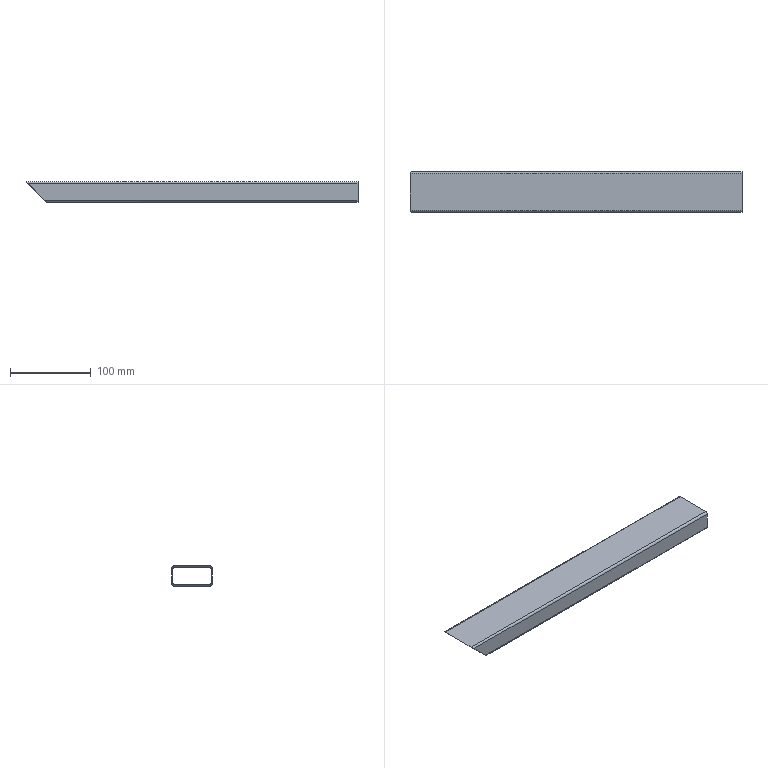Part | STEP file | 6150501 | 1 solid | 18 faces | box 410 x 50 x 25 mm | volume 84495 mm3 | plane 10 | cylinder 8 | commonest cylinder face diameters 3 x4 5 x4
STEP:
#1=CARTESIAN_POINT('',(205.,-25.,10.));
#2=VERTEX_POINT('',#1);
#3=CARTESIAN_POINT('',(-202.5,-25.,10.));
#4=VERTEX_POINT('',#3);
#5=CARTESIAN_POINT('',(-205.,-25.,10.));
#6=DIRECTION('',(-1.,0.,0.));
#7=VECTOR('',#6,1000.);
#8=LINE('',#5,#7);
#9=EDGE_CURVE('',#2,#4,#8,.T.);
#10=ORIENTED_EDGE('',*,*,#9,.T.);
#11=CARTESIAN_POINT('',(-182.5,-25.,-10.));
#12=VERTEX_POINT('',#11);
#13=CARTESIAN_POINT('',(-205.,-25.,12.5));
#14=DIRECTION('',(0.7071,0.,-0.7071));
#15=VECTOR('',#14,1000.);
#16=LINE('',#13,#15);
#17=EDGE_CURVE('',#4,#12,#16,.T.);
#18=ORIENTED_EDGE('',*,*,#17,.T.);
#19=CARTESIAN_POINT('',(205.,-25.,-10.));
#20=VERTEX_POINT('',#19);
#21=CARTESIAN_POINT('',(-205.,-25.,-10.));
#22=DIRECTION('',(1.,0.,0.));
#23=VECTOR('',#22,1000.);
#24=LINE('',#21,#23);
#25=EDGE_CURVE('',#12,#20,#24,.T.);
#26=ORIENTED_EDGE('',*,*,#25,.T.);
#27=CARTESIAN_POINT('',(205.,-25.,12.5));
#28=DIRECTION('',(0.,0.,-1.));
#29=VECTOR('',#28,1000.);
#30=LINE('',#27,#29);
#31=EDGE_CURVE('',#2,#20,#30,.T.);
#32=ORIENTED_EDGE('',*,*,#31,.F.);
#33=EDGE_LOOP('',(#10,#18,#26,#32));
#34=FACE_OUTER_BOUND('',#33,.T.);
#35=CARTESIAN_POINT('',(-205.,-25.,12.5));
#36=DIRECTION('',(0.,1.,0.));
#37=DIRECTION('',(-1.,0.,0.));
#38=AXIS2_PLACEMENT_3D('',#35,#36,#37);
#39=PLANE('',#38);
#40=ADVANCED_FACE('',(#34),#39,.F.);
#41=CARTESIAN_POINT('',(205.,-22.,-11.));
#42=VERTEX_POINT('',#41);
#43=CARTESIAN_POINT('',(205.,22.,-11.));
#44=VERTEX_POINT('',#43);
#45=CARTESIAN_POINT('',(205.,22.,-11.));
#46=DIRECTION('',(0.,1.,0.));
#47=VECTOR('',#46,1000.);
#48=LINE('',#45,#47);
#49=EDGE_CURVE('',#42,#44,#48,.T.);
#50=ORIENTED_EDGE('',*,*,#49,.F.);
#51=CARTESIAN_POINT('',(205.,-23.5,-9.5));
#52=VERTEX_POINT('',#51);
#53=CARTESIAN_POINT('',(205.,-22.,-9.5));
#54=DIRECTION('',(1.,0.,0.));
#55=DIRECTION('',(0.,0.,-1.));
#56=AXIS2_PLACEMENT_3D('',#53,#54,#55);
#57=CIRCLE('',#56,1.5);
#58=EDGE_CURVE('',#52,#42,#57,.T.);
#59=ORIENTED_EDGE('',*,*,#58,.F.);
#60=CARTESIAN_POINT('',(205.,-23.5,9.5));
#61=VERTEX_POINT('',#60);
#62=CARTESIAN_POINT('',(205.,-23.5,9.5));
#63=DIRECTION('',(0.,0.,-1.));
#64=VECTOR('',#63,1000.);
#65=LINE('',#62,#64);
#66=EDGE_CURVE('',#61,#52,#65,.T.);
#67=ORIENTED_EDGE('',*,*,#66,.F.);
#68=CARTESIAN_POINT('',(205.,-22.,11.));
#69=VERTEX_POINT('',#68);
#70=CARTESIAN_POINT('',(205.,-22.,9.5));
#71=DIRECTION('',(1.,0.,0.));
#72=DIRECTION('',(0.,0.,-1.));
#73=AXIS2_PLACEMENT_3D('',#70,#71,#72);
#74=CIRCLE('',#73,1.5);
#75=EDGE_CURVE('',#69,#61,#74,.T.);
#76=ORIENTED_EDGE('',*,*,#75,.F.);
#77=CARTESIAN_POINT('',(205.,22.,11.));
#78=VERTEX_POINT('',#77);
#79=CARTESIAN_POINT('',(205.,22.,11.));
#80=DIRECTION('',(0.,-1.,0.));
#81=VECTOR('',#80,1000.);
#82=LINE('',#79,#81);
#83=EDGE_CURVE('',#78,#69,#82,.T.);
#84=ORIENTED_EDGE('',*,*,#83,.F.);
#85=CARTESIAN_POINT('',(205.,23.5,9.5));
#86=VERTEX_POINT('',#85);
#87=CARTESIAN_POINT('',(205.,22.,9.5));
#88=DIRECTION('',(1.,0.,0.));
#89=DIRECTION('',(0.,0.,-1.));
#90=AXIS2_PLACEMENT_3D('',#87,#88,#89);
#91=CIRCLE('',#90,1.5);
#92=EDGE_CURVE('',#86,#78,#91,.T.);
#93=ORIENTED_EDGE('',*,*,#92,.F.);
#94=CARTESIAN_POINT('',(205.,23.5,-9.5));
#95=VERTEX_POINT('',#94);
#96=CARTESIAN_POINT('',(205.,23.5,9.5));
#97=DIRECTION('',(0.,0.,1.));
#98=VECTOR('',#97,1000.);
#99=LINE('',#96,#98);
#100=EDGE_CURVE('',#95,#86,#99,.T.);
#101=ORIENTED_EDGE('',*,*,#100,.F.);
#102=CARTESIAN_POINT('',(205.,22.,-9.5));
#103=DIRECTION('',(1.,0.,0.));
#104=DIRECTION('',(0.,0.,1.));
#105=AXIS2_PLACEMENT_3D('',#102,#103,#104);
#106=CIRCLE('',#105,1.5);
#107=EDGE_CURVE('',#44,#95,#106,.T.);
#108=ORIENTED_EDGE('',*,*,#107,.F.);
#109=EDGE_LOOP('',(#50,#59,#67,#76,#84,#93,#101,#108));
#110=FACE_BOUND('',#109,.T.);
#111=CARTESIAN_POINT('',(205.,-22.5,12.5));
#112=VERTEX_POINT('',#111);
#113=CARTESIAN_POINT('',(205.,22.5,12.5));
#114=VERTEX_POINT('',#113);
#115=CARTESIAN_POINT('',(205.,25.,12.5));
#116=DIRECTION('',(0.,1.,0.));
#117=VECTOR('',#116,1000.);
#118=LINE('',#115,#117);
#119=EDGE_CURVE('',#112,#114,#118,.T.);
#120=ORIENTED_EDGE('',*,*,#119,.F.);
#121=CARTESIAN_POINT('',(205.,-22.5,10.));
#122=DIRECTION('',(1.,0.,0.));
#123=DIRECTION('',(0.,0.,1.));
#124=AXIS2_PLACEMENT_3D('',#121,#122,#123);
#125=CIRCLE('',#124,2.5);
#126=EDGE_CURVE('',#112,#2,#125,.T.);
#127=ORIENTED_EDGE('',*,*,#126,.T.);
#128=ORIENTED_EDGE('',*,*,#31,.T.);
#129=CARTESIAN_POINT('',(205.,-22.5,-12.5));
#130=VERTEX_POINT('',#129);
#131=CARTESIAN_POINT('',(205.,-22.5,-10.));
#132=DIRECTION('',(1.,0.,0.));
#133=DIRECTION('',(0.,0.,1.));
#134=AXIS2_PLACEMENT_3D('',#131,#132,#133);
#135=CIRCLE('',#134,2.5);
#136=EDGE_CURVE('',#20,#130,#135,.T.);
#137=ORIENTED_EDGE('',*,*,#136,.T.);
#138=CARTESIAN_POINT('',(205.,22.5,-12.5));
#139=VERTEX_POINT('',#138);
#140=CARTESIAN_POINT('',(205.,25.,-12.5));
#141=DIRECTION('',(0.,1.,0.));
#142=VECTOR('',#141,1000.);
#143=LINE('',#140,#142);
#144=EDGE_CURVE('',#130,#139,#143,.T.);
#145=ORIENTED_EDGE('',*,*,#144,.T.);
#146=CARTESIAN_POINT('',(205.,25.,-10.));
#147=VERTEX_POINT('',#146);
#148=CARTESIAN_POINT('',(205.,22.5,-10.));
#149=DIRECTION('',(1.,0.,0.));
#150=DIRECTION('',(0.,0.,1.));
#151=AXIS2_PLACEMENT_3D('',#148,#149,#150);
#152=CIRCLE('',#151,2.5);
#153=EDGE_CURVE('',#139,#147,#152,.T.);
#154=ORIENTED_EDGE('',*,*,#153,.T.);
#155=CARTESIAN_POINT('',(205.,25.,10.));
#156=VERTEX_POINT('',#155);
#157=CARTESIAN_POINT('',(205.,25.,12.5));
#158=DIRECTION('',(0.,0.,-1.));
#159=VECTOR('',#158,1000.);
#160=LINE('',#157,#159);
#161=EDGE_CURVE('',#156,#147,#160,.T.);
#162=ORIENTED_EDGE('',*,*,#161,.F.);
#163=CARTESIAN_POINT('',(205.,22.5,10.));
#164=DIRECTION('',(1.,0.,0.));
#165=DIRECTION('',(0.,0.,1.));
#166=AXIS2_PLACEMENT_3D('',#163,#164,#165);
#167=CIRCLE('',#166,2.5);
#168=EDGE_CURVE('',#156,#114,#167,.T.);
#169=ORIENTED_EDGE('',*,*,#168,.T.);
#170=EDGE_LOOP('',(#120,#127,#128,#137,#145,#154,#162,#169));
#171=FACE_OUTER_BOUND('',#170,.T.);
#172=CARTESIAN_POINT('',(205.,25.,12.5));
#173=DIRECTION('',(-1.,0.,0.));
#174=DIRECTION('',(0.,0.,1.));
#175=AXIS2_PLACEMENT_3D('',#172,#173,#174);
#176=PLANE('',#175);
#177=ADVANCED_FACE('',(#110,#171),#176,.F.);
#178=CARTESIAN_POINT('',(-182.5,25.,-10.));
#179=VERTEX_POINT('',#178);
#180=CARTESIAN_POINT('',(-205.,25.,-10.));
#181=DIRECTION('',(-1.,0.,0.));
#182=VECTOR('',#181,1000.);
#183=LINE('',#180,#182);
#184=EDGE_CURVE('',#147,#179,#183,.T.);
#185=ORIENTED_EDGE('',*,*,#184,.T.);
#186=CARTESIAN_POINT('',(-202.5,25.,10.));
#187=VERTEX_POINT('',#186);
#188=CARTESIAN_POINT('',(-205.,25.,12.5));
#189=DIRECTION('',(0.7071,0.,-0.7071));
#190=VECTOR('',#189,1000.);
#191=LINE('',#188,#190);
#192=EDGE_CURVE('',#187,#179,#191,.T.);
#193=ORIENTED_EDGE('',*,*,#192,.F.);
#194=CARTESIAN_POINT('',(205.,25.,10.));
#195=DIRECTION('',(1.,0.,0.));
#196=VECTOR('',#195,1000.);
#197=LINE('',#194,#196);
#198=EDGE_CURVE('',#187,#156,#197,.T.);
#199=ORIENTED_EDGE('',*,*,#198,.T.);
#200=ORIENTED_EDGE('',*,*,#161,.T.);
#201=EDGE_LOOP('',(#185,#193,#199,#200));
#202=FACE_OUTER_BOUND('',#201,.T.);
#203=CARTESIAN_POINT('',(-205.,25.,12.5));
#204=DIRECTION('',(0.,-1.,0.));
#205=DIRECTION('',(0.,0.,-1.));
#206=AXIS2_PLACEMENT_3D('',#203,#204,#205);
#207=PLANE('',#206);
#208=ADVANCED_FACE('',(#202),#207,.F.);
#209=CARTESIAN_POINT('',(-205.,22.5,12.5));
#210=VERTEX_POINT('',#209);
#211=CARTESIAN_POINT('',(-205.,-22.5,12.5));
#212=VERTEX_POINT('',#211);
#213=CARTESIAN_POINT('',(-205.,25.,12.5));
#214=DIRECTION('',(0.,-1.,0.));
#215=VECTOR('',#214,1000.);
#216=LINE('',#213,#215);
#217=EDGE_CURVE('',#210,#212,#216,.T.);
#218=ORIENTED_EDGE('',*,*,#217,.T.);
#219=CARTESIAN_POINT('',(205.,-22.5,12.5));
#220=DIRECTION('',(1.,0.,0.));
#221=VECTOR('',#220,1000.);
#222=LINE('',#219,#221);
#223=EDGE_CURVE('',#212,#112,#222,.T.);
#224=ORIENTED_EDGE('',*,*,#223,.T.);
#225=ORIENTED_EDGE('',*,*,#119,.T.);
#226=CARTESIAN_POINT('',(-205.,22.5,12.5));
#227=DIRECTION('',(-1.,0.,0.));
#228=VECTOR('',#227,1000.);
#229=LINE('',#226,#228);
#230=EDGE_CURVE('',#114,#210,#229,.T.);
#231=ORIENTED_EDGE('',*,*,#230,.T.);
#232=EDGE_LOOP('',(#218,#224,#225,#231));
#233=FACE_OUTER_BOUND('',#232,.T.);
#234=CARTESIAN_POINT('',(-205.,25.,12.5));
#235=DIRECTION('',(0.,0.,1.));
#236=DIRECTION('',(1.,0.,0.));
#237=AXIS2_PLACEMENT_3D('',#234,#235,#236);
#238=PLANE('',#237);
#239=ADVANCED_FACE('',(#233),#238,.T.);
#240=CARTESIAN_POINT('',(-180.,-22.5,-12.5));
#241=VERTEX_POINT('',#240);
#242=CARTESIAN_POINT('',(-205.,-22.5,-12.5));
#243=DIRECTION('',(-1.,0.,0.));
#244=VECTOR('',#243,1000.);
#245=LINE('',#242,#244);
#246=EDGE_CURVE('',#130,#241,#245,.T.);
#247=ORIENTED_EDGE('',*,*,#246,.T.);
#248=CARTESIAN_POINT('',(-180.,22.5,-12.5));
#249=VERTEX_POINT('',#248);
#250=CARTESIAN_POINT('',(-180.,-25.,-12.5));
#251=DIRECTION('',(0.,1.,0.));
#252=VECTOR('',#251,1000.);
#253=LINE('',#250,#252);
#254=EDGE_CURVE('',#241,#249,#253,.T.);
#255=ORIENTED_EDGE('',*,*,#254,.T.);
#256=CARTESIAN_POINT('',(-205.,22.5,-12.5));
#257=DIRECTION('',(1.,0.,0.));
#258=VECTOR('',#257,1000.);
#259=LINE('',#256,#258);
#260=EDGE_CURVE('',#249,#139,#259,.T.);
#261=ORIENTED_EDGE('',*,*,#260,.T.);
#262=ORIENTED_EDGE('',*,*,#144,.F.);
#263=EDGE_LOOP('',(#247,#255,#261,#262));
#264=FACE_OUTER_BOUND('',#263,.T.);
#265=CARTESIAN_POINT('',(-205.,25.,-12.5));
#266=DIRECTION('',(0.,0.,1.));
#267=DIRECTION('',(1.,0.,0.));
#268=AXIS2_PLACEMENT_3D('',#265,#266,#267);
#269=PLANE('',#268);
#270=ADVANCED_FACE('',(#264),#269,.F.);
#271=CARTESIAN_POINT('',(-202.5,-25.,10.));
#272=CARTESIAN_POINT('',(-203.964,-25.,11.464));
#273=CARTESIAN_POINT('',(-205.,-23.964,12.5));
#274=CARTESIAN_POINT('',(-205.,-22.5,12.5));
#275=(BOUNDED_CURVE()B_SPLINE_CURVE(3,(#271,#272,#273,#274),.UNSPECIFIED.,.F.,.T.)B_SPLINE_CURVE_WITH_KNOTS((4,4),(4.712,6.283),.UNSPECIFIED.)CURVE()GEOMETRIC_REPRESENTATION_ITEM()RATIONAL_B_SPLINE_CURVE((1.,0.8047,0.8047,1.))REPRESENTATION_ITEM(''));
#276=EDGE_CURVE('',#4,#212,#275,.T.);
#277=ORIENTED_EDGE('',*,*,#276,.F.);
#278=ORIENTED_EDGE('',*,*,#9,.F.);
#279=ORIENTED_EDGE('',*,*,#126,.F.);
#280=ORIENTED_EDGE('',*,*,#223,.F.);
#281=EDGE_LOOP('',(#277,#278,#279,#280));
#282=FACE_OUTER_BOUND('',#281,.T.);
#283=CARTESIAN_POINT('',(-205.,-22.5,10.));
#284=DIRECTION('',(-1.,0.,0.));
#285=DIRECTION('',(0.,-1.,0.));
#286=AXIS2_PLACEMENT_3D('',#283,#284,#285);
#287=CYLINDRICAL_SURFACE('',#286,2.5);
#288=ADVANCED_FACE('',(#282),#287,.T.);
#289=CARTESIAN_POINT('',(-180.,-22.5,-12.5));
#290=CARTESIAN_POINT('',(-180.,-23.964,-12.5));
#291=CARTESIAN_POINT('',(-181.036,-25.,-11.464));
#292=CARTESIAN_POINT('',(-182.5,-25.,-10.));
#293=(BOUNDED_CURVE()B_SPLINE_CURVE(3,(#289,#290,#291,#292),.UNSPECIFIED.,.F.,.F.)B_SPLINE_CURVE_WITH_KNOTS((4,4),(0.,1.571),.UNSPECIFIED.)CURVE()GEOMETRIC_REPRESENTATION_ITEM()RATIONAL_B_SPLINE_CURVE((1.,0.8047,0.8047,1.))REPRESENTATION_ITEM(''));
#294=EDGE_CURVE('',#241,#12,#293,.T.);
#295=ORIENTED_EDGE('',*,*,#294,.F.);
#296=ORIENTED_EDGE('',*,*,#246,.F.);
#297=ORIENTED_EDGE('',*,*,#136,.F.);
#298=ORIENTED_EDGE('',*,*,#25,.F.);
#299=EDGE_LOOP('',(#295,#296,#297,#298));
#300=FACE_OUTER_BOUND('',#299,.T.);
#301=CARTESIAN_POINT('',(-205.,-22.5,-10.));
#302=DIRECTION('',(1.,0.,0.));
#303=DIRECTION('',(0.,1.,0.));
#304=AXIS2_PLACEMENT_3D('',#301,#302,#303);
#305=CYLINDRICAL_SURFACE('',#304,2.5);
#306=ADVANCED_FACE('',(#300),#305,.T.);
#307=CARTESIAN_POINT('',(-182.5,25.,-10.));
#308=CARTESIAN_POINT('',(-181.036,25.,-11.464));
#309=CARTESIAN_POINT('',(-180.,23.964,-12.5));
#310=CARTESIAN_POINT('',(-180.,22.5,-12.5));
#311=(BOUNDED_CURVE()B_SPLINE_CURVE(3,(#307,#308,#309,#310),.UNSPECIFIED.,.F.,.F.)B_SPLINE_CURVE_WITH_KNOTS((4,4),(1.571,3.142),.UNSPECIFIED.)CURVE()GEOMETRIC_REPRESENTATION_ITEM()RATIONAL_B_SPLINE_CURVE((1.,0.8047,0.8047,1.))REPRESENTATION_ITEM(''));
#312=EDGE_CURVE('',#179,#249,#311,.T.);
#313=ORIENTED_EDGE('',*,*,#312,.F.);
#314=ORIENTED_EDGE('',*,*,#184,.F.);
#315=ORIENTED_EDGE('',*,*,#153,.F.);
#316=ORIENTED_EDGE('',*,*,#260,.F.);
#317=EDGE_LOOP('',(#313,#314,#315,#316));
#318=FACE_OUTER_BOUND('',#317,.T.);
#319=CARTESIAN_POINT('',(-205.,22.5,-10.));
#320=DIRECTION('',(-1.,0.,0.));
#321=DIRECTION('',(0.,0.,1.));
#322=AXIS2_PLACEMENT_3D('',#319,#320,#321);
#323=CYLINDRICAL_SURFACE('',#322,2.5);
#324=ADVANCED_FACE('',(#318),#323,.T.);
#325=CARTESIAN_POINT('',(-205.,22.5,12.5));
#326=CARTESIAN_POINT('',(-205.,23.964,12.5));
#327=CARTESIAN_POINT('',(-203.964,25.,11.464));
#328=CARTESIAN_POINT('',(-202.5,25.,10.));
#329=(BOUNDED_CURVE()B_SPLINE_CURVE(3,(#325,#326,#327,#328),.UNSPECIFIED.,.F.,.F.)B_SPLINE_CURVE_WITH_KNOTS((4,4),(3.142,4.712),.UNSPECIFIED.)CURVE()GEOMETRIC_REPRESENTATION_ITEM()RATIONAL_B_SPLINE_CURVE((1.,0.8047,0.8047,1.))REPRESENTATION_ITEM(''));
#330=EDGE_CURVE('',#210,#187,#329,.T.);
#331=ORIENTED_EDGE('',*,*,#330,.F.);
#332=ORIENTED_EDGE('',*,*,#230,.F.);
#333=ORIENTED_EDGE('',*,*,#168,.F.);
#334=ORIENTED_EDGE('',*,*,#198,.F.);
#335=EDGE_LOOP('',(#331,#332,#333,#334));
#336=FACE_OUTER_BOUND('',#335,.T.);
#337=CARTESIAN_POINT('',(-205.,22.5,10.));
#338=DIRECTION('',(1.,0.,0.));
#339=DIRECTION('',(0.,0.,-1.));
#340=AXIS2_PLACEMENT_3D('',#337,#338,#339);
#341=CYLINDRICAL_SURFACE('',#340,2.5);
#342=ADVANCED_FACE('',(#336),#341,.T.);
#343=CARTESIAN_POINT('',(-202.,-23.5,9.5));
#344=VERTEX_POINT('',#343);
#345=CARTESIAN_POINT('',(-183.,-23.5,-9.5));
#346=VERTEX_POINT('',#345);
#347=CARTESIAN_POINT('',(-205.,-23.5,12.5));
#348=DIRECTION('',(0.7071,0.,-0.7071));
#349=VECTOR('',#348,1000.);
#350=LINE('',#347,#349);
#351=EDGE_CURVE('',#344,#346,#350,.T.);
#352=ORIENTED_EDGE('',*,*,#351,.T.);
#353=CARTESIAN_POINT('',(-181.5,-22.,-11.));
#354=VERTEX_POINT('',#353);
#355=CARTESIAN_POINT('',(-183.,-23.5,-9.5));
#356=CARTESIAN_POINT('',(-182.121,-23.5,-10.379));
#357=CARTESIAN_POINT('',(-181.5,-22.879,-11.));
#358=CARTESIAN_POINT('',(-181.5,-22.,-11.));
#359=(BOUNDED_CURVE()B_SPLINE_CURVE(3,(#355,#356,#357,#358),.UNSPECIFIED.,.F.,.F.)B_SPLINE_CURVE_WITH_KNOTS((4,4),(4.712,6.283),.UNSPECIFIED.)CURVE()GEOMETRIC_REPRESENTATION_ITEM()RATIONAL_B_SPLINE_CURVE((1.,0.8047,0.8047,1.))REPRESENTATION_ITEM(''));
#360=EDGE_CURVE('',#346,#354,#359,.T.);
#361=ORIENTED_EDGE('',*,*,#360,.T.);
#362=CARTESIAN_POINT('',(-181.5,22.,-11.));
#363=VERTEX_POINT('',#362);
#364=CARTESIAN_POINT('',(-181.5,-25.,-11.));
#365=DIRECTION('',(0.,1.,0.));
#366=VECTOR('',#365,1000.);
#367=LINE('',#364,#366);
#368=EDGE_CURVE('',#354,#363,#367,.T.);
#369=ORIENTED_EDGE('',*,*,#368,.T.);
#370=CARTESIAN_POINT('',(-183.,23.5,-9.5));
#371=VERTEX_POINT('',#370);
#372=CARTESIAN_POINT('',(-181.5,22.,-11.));
#373=CARTESIAN_POINT('',(-181.5,22.879,-11.));
#374=CARTESIAN_POINT('',(-182.121,23.5,-10.379));
#375=CARTESIAN_POINT('',(-183.,23.5,-9.5));
#376=(BOUNDED_CURVE()B_SPLINE_CURVE(3,(#372,#373,#374,#375),.UNSPECIFIED.,.F.,.T.)B_SPLINE_CURVE_WITH_KNOTS((4,4),(0.,1.571),.UNSPECIFIED.)CURVE()GEOMETRIC_REPRESENTATION_ITEM()RATIONAL_B_SPLINE_CURVE((1.,0.8047,0.8047,1.))REPRESENTATION_ITEM(''));
#377=EDGE_CURVE('',#363,#371,#376,.T.);
#378=ORIENTED_EDGE('',*,*,#377,.T.);
#379=CARTESIAN_POINT('',(-202.,23.5,9.5));
#380=VERTEX_POINT('',#379);
#381=CARTESIAN_POINT('',(-205.,23.5,12.5));
#382=DIRECTION('',(-0.7071,0.,0.7071));
#383=VECTOR('',#382,1000.);
#384=LINE('',#381,#383);
#385=EDGE_CURVE('',#371,#380,#384,.T.);
#386=ORIENTED_EDGE('',*,*,#385,.T.);
#387=CARTESIAN_POINT('',(-203.5,22.,11.));
#388=VERTEX_POINT('',#387);
#389=CARTESIAN_POINT('',(-202.,23.5,9.5));
#390=CARTESIAN_POINT('',(-202.879,23.5,10.379));
#391=CARTESIAN_POINT('',(-203.5,22.879,11.));
#392=CARTESIAN_POINT('',(-203.5,22.,11.));
#393=(BOUNDED_CURVE()B_SPLINE_CURVE(3,(#389,#390,#391,#392),.UNSPECIFIED.,.F.,.F.)B_SPLINE_CURVE_WITH_KNOTS((4,4),(1.571,3.142),.UNSPECIFIED.)CURVE()GEOMETRIC_REPRESENTATION_ITEM()RATIONAL_B_SPLINE_CURVE((1.,0.8047,0.8047,1.))REPRESENTATION_ITEM(''));
#394=EDGE_CURVE('',#380,#388,#393,.T.);
#395=ORIENTED_EDGE('',*,*,#394,.T.);
#396=CARTESIAN_POINT('',(-203.5,-22.,11.));
#397=VERTEX_POINT('',#396);
#398=CARTESIAN_POINT('',(-203.5,-25.,11.));
#399=DIRECTION('',(0.,-1.,0.));
#400=VECTOR('',#399,1000.);
#401=LINE('',#398,#400);
#402=EDGE_CURVE('',#388,#397,#401,.T.);
#403=ORIENTED_EDGE('',*,*,#402,.T.);
#404=CARTESIAN_POINT('',(-203.5,-22.,11.));
#405=CARTESIAN_POINT('',(-203.5,-22.879,11.));
#406=CARTESIAN_POINT('',(-202.879,-23.5,10.379));
#407=CARTESIAN_POINT('',(-202.,-23.5,9.5));
#408=(BOUNDED_CURVE()B_SPLINE_CURVE(3,(#404,#405,#406,#407),.UNSPECIFIED.,.F.,.F.)B_SPLINE_CURVE_WITH_KNOTS((4,4),(3.142,4.712),.UNSPECIFIED.)CURVE()GEOMETRIC_REPRESENTATION_ITEM()RATIONAL_B_SPLINE_CURVE((1.,0.8047,0.8047,1.))REPRESENTATION_ITEM(''));
#409=EDGE_CURVE('',#397,#344,#408,.T.);
#410=ORIENTED_EDGE('',*,*,#409,.T.);
#411=EDGE_LOOP('',(#352,#361,#369,#378,#386,#395,#403,#410));
#412=FACE_BOUND('',#411,.T.);
#413=ORIENTED_EDGE('',*,*,#276,.T.);
#414=ORIENTED_EDGE('',*,*,#217,.F.);
#415=ORIENTED_EDGE('',*,*,#330,.T.);
#416=ORIENTED_EDGE('',*,*,#192,.T.);
#417=ORIENTED_EDGE('',*,*,#312,.T.);
#418=ORIENTED_EDGE('',*,*,#254,.F.);
#419=ORIENTED_EDGE('',*,*,#294,.T.);
#420=ORIENTED_EDGE('',*,*,#17,.F.);
#421=EDGE_LOOP('',(#413,#414,#415,#416,#417,#418,#419,#420));
#422=FACE_OUTER_BOUND('',#421,.T.);
#423=CARTESIAN_POINT('',(-205.,-25.,12.5));
#424=DIRECTION('',(0.7071,0.,0.7071));
#425=DIRECTION('',(0.7071,0.,-0.7071));
#426=AXIS2_PLACEMENT_3D('',#423,#424,#425);
#427=PLANE('',#426);
#428=ADVANCED_FACE('',(#412,#422),#427,.F.);
#429=CARTESIAN_POINT('',(-205.,-23.5,-9.5));
#430=DIRECTION('',(1.,0.,0.));
#431=VECTOR('',#430,1000.);
#432=LINE('',#429,#431);
#433=EDGE_CURVE('',#346,#52,#432,.T.);
#434=ORIENTED_EDGE('',*,*,#433,.T.);
#435=ORIENTED_EDGE('',*,*,#58,.T.);
#436=CARTESIAN_POINT('',(-205.,-22.,-11.));
#437=DIRECTION('',(1.,0.,0.));
#438=VECTOR('',#437,1000.);
#439=LINE('',#436,#438);
#440=EDGE_CURVE('',#354,#42,#439,.T.);
#441=ORIENTED_EDGE('',*,*,#440,.F.);
#442=ORIENTED_EDGE('',*,*,#360,.F.);
#443=EDGE_LOOP('',(#434,#435,#441,#442));
#444=FACE_OUTER_BOUND('',#443,.T.);
#445=CARTESIAN_POINT('',(-205.,-22.,-9.5));
#446=DIRECTION('',(1.,0.,0.));
#447=DIRECTION('',(0.,0.,-1.));
#448=AXIS2_PLACEMENT_3D('',#445,#446,#447);
#449=CYLINDRICAL_SURFACE('',#448,1.5);
#450=ADVANCED_FACE('',(#444),#449,.F.);
#451=CARTESIAN_POINT('',(-205.,-23.5,9.5));
#452=DIRECTION('',(1.,0.,0.));
#453=VECTOR('',#452,1000.);
#454=LINE('',#451,#453);
#455=EDGE_CURVE('',#344,#61,#454,.T.);
#456=ORIENTED_EDGE('',*,*,#455,.T.);
#457=ORIENTED_EDGE('',*,*,#66,.T.);
#458=ORIENTED_EDGE('',*,*,#433,.F.);
#459=ORIENTED_EDGE('',*,*,#351,.F.);
#460=EDGE_LOOP('',(#456,#457,#458,#459));
#461=FACE_OUTER_BOUND('',#460,.T.);
#462=CARTESIAN_POINT('',(-205.,-23.5,9.5));
#463=DIRECTION('',(0.,-1.,0.));
#464=DIRECTION('',(0.,0.,-1.));
#465=AXIS2_PLACEMENT_3D('',#462,#463,#464);
#466=PLANE('',#465);
#467=ADVANCED_FACE('',(#461),#466,.F.);
#468=CARTESIAN_POINT('',(-205.,-22.,11.));
#469=DIRECTION('',(1.,0.,0.));
#470=VECTOR('',#469,1000.);
#471=LINE('',#468,#470);
#472=EDGE_CURVE('',#397,#69,#471,.T.);
#473=ORIENTED_EDGE('',*,*,#472,.T.);
#474=ORIENTED_EDGE('',*,*,#75,.T.);
#475=ORIENTED_EDGE('',*,*,#455,.F.);
#476=ORIENTED_EDGE('',*,*,#409,.F.);
#477=EDGE_LOOP('',(#473,#474,#475,#476));
#478=FACE_OUTER_BOUND('',#477,.T.);
#479=CARTESIAN_POINT('',(-205.,-22.,9.5));
#480=DIRECTION('',(1.,0.,0.));
#481=DIRECTION('',(0.,0.,-1.));
#482=AXIS2_PLACEMENT_3D('',#479,#480,#481);
#483=CYLINDRICAL_SURFACE('',#482,1.5);
#484=ADVANCED_FACE('',(#478),#483,.F.);
#485=CARTESIAN_POINT('',(-205.,22.,11.));
#486=DIRECTION('',(1.,0.,0.));
#487=VECTOR('',#486,1000.);
#488=LINE('',#485,#487);
#489=EDGE_CURVE('',#388,#78,#488,.T.);
#490=ORIENTED_EDGE('',*,*,#489,.T.);
#491=ORIENTED_EDGE('',*,*,#83,.T.);
#492=ORIENTED_EDGE('',*,*,#472,.F.);
#493=ORIENTED_EDGE('',*,*,#402,.F.);
#494=EDGE_LOOP('',(#490,#491,#492,#493));
#495=FACE_OUTER_BOUND('',#494,.T.);
#496=CARTESIAN_POINT('',(-205.,22.,11.));
#497=DIRECTION('',(0.,0.,1.));
#498=DIRECTION('',(0.,-1.,0.));
#499=AXIS2_PLACEMENT_3D('',#496,#497,#498);
#500=PLANE('',#499);
#501=ADVANCED_FACE('',(#495),#500,.F.);
#502=CARTESIAN_POINT('',(-205.,23.5,9.5));
#503=DIRECTION('',(1.,0.,0.));
#504=VECTOR('',#503,1000.);
#505=LINE('',#502,#504);
#506=EDGE_CURVE('',#380,#86,#505,.T.);
#507=ORIENTED_EDGE('',*,*,#506,.T.);
#508=ORIENTED_EDGE('',*,*,#92,.T.);
#509=ORIENTED_EDGE('',*,*,#489,.F.);
#510=ORIENTED_EDGE('',*,*,#394,.F.);
#511=EDGE_LOOP('',(#507,#508,#509,#510));
#512=FACE_OUTER_BOUND('',#511,.T.);
#513=CARTESIAN_POINT('',(-205.,22.,9.5));
#514=DIRECTION('',(1.,0.,0.));
#515=DIRECTION('',(0.,0.,-1.));
#516=AXIS2_PLACEMENT_3D('',#513,#514,#515);
#517=CYLINDRICAL_SURFACE('',#516,1.5);
#518=ADVANCED_FACE('',(#512),#517,.F.);
#519=CARTESIAN_POINT('',(-205.,23.5,-9.5));
#520=DIRECTION('',(1.,0.,0.));
#521=VECTOR('',#520,1000.);
#522=LINE('',#519,#521);
#523=EDGE_CURVE('',#371,#95,#522,.T.);
#524=ORIENTED_EDGE('',*,*,#523,.T.);
#525=ORIENTED_EDGE('',*,*,#100,.T.);
#526=ORIENTED_EDGE('',*,*,#506,.F.);
#527=ORIENTED_EDGE('',*,*,#385,.F.);
#528=EDGE_LOOP('',(#524,#525,#526,#527));
#529=FACE_OUTER_BOUND('',#528,.T.);
#530=CARTESIAN_POINT('',(-205.,23.5,9.5));
#531=DIRECTION('',(0.,1.,0.));
#532=DIRECTION('',(0.,0.,1.));
#533=AXIS2_PLACEMENT_3D('',#530,#531,#532);
#534=PLANE('',#533);
#535=ADVANCED_FACE('',(#529),#534,.F.);
#536=CARTESIAN_POINT('',(-205.,22.,-11.));
#537=DIRECTION('',(1.,0.,0.));
#538=VECTOR('',#537,1000.);
#539=LINE('',#536,#538);
#540=EDGE_CURVE('',#363,#44,#539,.T.);
#541=ORIENTED_EDGE('',*,*,#540,.T.);
#542=ORIENTED_EDGE('',*,*,#107,.T.);
#543=ORIENTED_EDGE('',*,*,#523,.F.);
#544=ORIENTED_EDGE('',*,*,#377,.F.);
#545=EDGE_LOOP('',(#541,#542,#543,#544));
#546=FACE_OUTER_BOUND('',#545,.T.);
#547=CARTESIAN_POINT('',(-205.,22.,-9.5));
#548=DIRECTION('',(1.,0.,0.));
#549=DIRECTION('',(0.,0.,-1.));
#550=AXIS2_PLACEMENT_3D('',#547,#548,#549);
#551=CYLINDRICAL_SURFACE('',#550,1.5);
#552=ADVANCED_FACE('',(#546),#551,.F.);
#553=ORIENTED_EDGE('',*,*,#440,.T.);
#554=ORIENTED_EDGE('',*,*,#49,.T.);
#555=ORIENTED_EDGE('',*,*,#540,.F.);
#556=ORIENTED_EDGE('',*,*,#368,.F.);
#557=EDGE_LOOP('',(#553,#554,#555,#556));
#558=FACE_OUTER_BOUND('',#557,.T.);
#559=CARTESIAN_POINT('',(-205.,22.,-11.));
#560=DIRECTION('',(0.,0.,-1.));
#561=DIRECTION('',(0.,1.,0.));
#562=AXIS2_PLACEMENT_3D('',#559,#560,#561);
#563=PLANE('',#562);
#564=ADVANCED_FACE('',(#558),#563,.F.);
#565=CLOSED_SHELL('',(#40,#177,#208,#239,#270,#288,#306,#324,#342,#428,#450,#467,#484,#501,#518,#535,#552,#564));
#566=MANIFOLD_SOLID_BREP('',#565);
#567=CARTESIAN_POINT('',(0.,0.,0.));
#568=DIRECTION('',(0.,0.,1.));
#569=DIRECTION('',(1.,0.,0.));
#570=AXIS2_PLACEMENT_3D('',#567,#568,#569);
#571=(LENGTH_UNIT()NAMED_UNIT(*)SI_UNIT(.MILLI.,.METRE.));
#572=UNCERTAINTY_MEASURE_WITH_UNIT(LENGTH_MEASURE(0.00001),#571,'','');
#573=(NAMED_UNIT(*)PLANE_ANGLE_UNIT()SI_UNIT($,.RADIAN.));
#574=(NAMED_UNIT(*)SI_UNIT($,.STERADIAN.)SOLID_ANGLE_UNIT());
#575=(GEOMETRIC_REPRESENTATION_CONTEXT(3)GLOBAL_UNCERTAINTY_ASSIGNED_CONTEXT((#572))GLOBAL_UNIT_ASSIGNED_CONTEXT((#571,#573,#574))REPRESENTATION_CONTEXT('',''));
#576=ADVANCED_BREP_SHAPE_REPRESENTATION('',(#566,#570),#575);